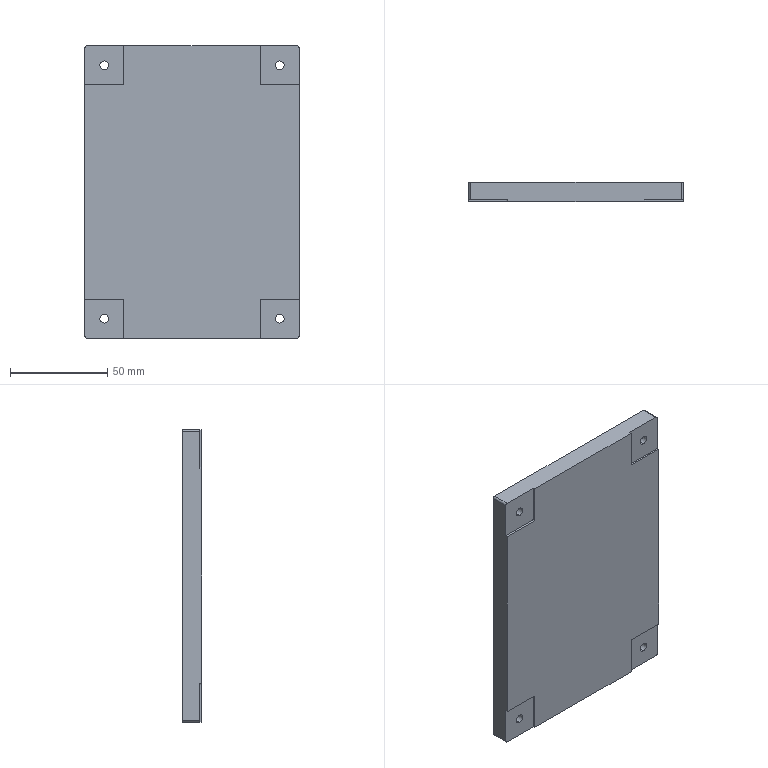Part | SolidWorks | features Fillet 2, Extrusion 1, HoleWzd 1, ICE 1 | 1 solid | 34 faces | box 110 x 10 x 150 mm | volume 162821 mm3 | plane 18 | cylinder 16 | commonest cylinder face diameters 2 x8 4.5 x8
STEP:
#1=CARTESIAN_POINT('',(45.,10.,-62.75));
#2=VERTEX_POINT('',#1);
#3=CARTESIAN_POINT('',(45.,10.,-67.25));
#4=VERTEX_POINT('',#3);
#5=CARTESIAN_POINT('',(45.,10.,-65.));
#6=DIRECTION('',(0.,-1.,0.));
#7=DIRECTION('',(0.,0.,-1.));
#8=AXIS2_PLACEMENT_3D('',#5,#6,#7);
#9=CIRCLE('',#8,2.25);
#10=EDGE_CURVE('',#2,#4,#9,.T.);
#11=ORIENTED_EDGE('',*,*,#10,.F.);
#12=CARTESIAN_POINT('',(45.,1.,-62.75));
#13=VERTEX_POINT('',#12);
#14=CARTESIAN_POINT('',(45.,1.,-62.75));
#15=DIRECTION('',(0.,-1.,0.));
#16=VECTOR('',#15,1000.);
#17=LINE('',#14,#16);
#18=EDGE_CURVE('',#2,#13,#17,.T.);
#19=ORIENTED_EDGE('',*,*,#18,.T.);
#20=CARTESIAN_POINT('',(45.,1.,-67.25));
#21=VERTEX_POINT('',#20);
#22=CARTESIAN_POINT('',(45.,1.,-65.));
#23=DIRECTION('',(0.,-1.,0.));
#24=DIRECTION('',(0.,0.,-1.));
#25=AXIS2_PLACEMENT_3D('',#22,#23,#24);
#26=CIRCLE('',#25,2.25);
#27=EDGE_CURVE('',#13,#21,#26,.T.);
#28=ORIENTED_EDGE('',*,*,#27,.T.);
#29=CARTESIAN_POINT('',(45.,1.,-67.25));
#30=DIRECTION('',(0.,-1.,0.));
#31=VECTOR('',#30,1000.);
#32=LINE('',#29,#31);
#33=EDGE_CURVE('',#4,#21,#32,.T.);
#34=ORIENTED_EDGE('',*,*,#33,.F.);
#35=EDGE_LOOP('',(#11,#19,#28,#34));
#36=FACE_OUTER_BOUND('',#35,.T.);
#37=CARTESIAN_POINT('',(45.,1.,-65.));
#38=DIRECTION('',(0.,-1.,0.));
#39=DIRECTION('',(0.,0.,-1.));
#40=AXIS2_PLACEMENT_3D('',#37,#38,#39);
#41=CYLINDRICAL_SURFACE('',#40,2.25);
#42=ADVANCED_FACE('',(#36),#41,.F.);
#43=CARTESIAN_POINT('',(-45.,10.,-62.75));
#44=VERTEX_POINT('',#43);
#45=CARTESIAN_POINT('',(-45.,10.,-67.25));
#46=VERTEX_POINT('',#45);
#47=CARTESIAN_POINT('',(-45.,10.,-65.));
#48=DIRECTION('',(0.,-1.,0.));
#49=DIRECTION('',(0.,0.,-1.));
#50=AXIS2_PLACEMENT_3D('',#47,#48,#49);
#51=CIRCLE('',#50,2.25);
#52=EDGE_CURVE('',#44,#46,#51,.T.);
#53=ORIENTED_EDGE('',*,*,#52,.F.);
#54=CARTESIAN_POINT('',(-45.,1.,-62.75));
#55=VERTEX_POINT('',#54);
#56=CARTESIAN_POINT('',(-45.,1.,-62.75));
#57=DIRECTION('',(0.,-1.,0.));
#58=VECTOR('',#57,1000.);
#59=LINE('',#56,#58);
#60=EDGE_CURVE('',#44,#55,#59,.T.);
#61=ORIENTED_EDGE('',*,*,#60,.T.);
#62=CARTESIAN_POINT('',(-45.,1.,-67.25));
#63=VERTEX_POINT('',#62);
#64=CARTESIAN_POINT('',(-45.,1.,-65.));
#65=DIRECTION('',(0.,-1.,0.));
#66=DIRECTION('',(0.,0.,-1.));
#67=AXIS2_PLACEMENT_3D('',#64,#65,#66);
#68=CIRCLE('',#67,2.25);
#69=EDGE_CURVE('',#55,#63,#68,.T.);
#70=ORIENTED_EDGE('',*,*,#69,.T.);
#71=CARTESIAN_POINT('',(-45.,1.,-67.25));
#72=DIRECTION('',(0.,-1.,0.));
#73=VECTOR('',#72,1000.);
#74=LINE('',#71,#73);
#75=EDGE_CURVE('',#46,#63,#74,.T.);
#76=ORIENTED_EDGE('',*,*,#75,.F.);
#77=EDGE_LOOP('',(#53,#61,#70,#76));
#78=FACE_OUTER_BOUND('',#77,.T.);
#79=CARTESIAN_POINT('',(-45.,1.,-65.));
#80=DIRECTION('',(0.,-1.,0.));
#81=DIRECTION('',(0.,0.,-1.));
#82=AXIS2_PLACEMENT_3D('',#79,#80,#81);
#83=CYLINDRICAL_SURFACE('',#82,2.25);
#84=ADVANCED_FACE('',(#78),#83,.F.);
#85=CARTESIAN_POINT('',(-45.,10.,67.25));
#86=VERTEX_POINT('',#85);
#87=CARTESIAN_POINT('',(-45.,10.,62.75));
#88=VERTEX_POINT('',#87);
#89=CARTESIAN_POINT('',(-45.,10.,65.));
#90=DIRECTION('',(0.,-1.,0.));
#91=DIRECTION('',(0.,0.,-1.));
#92=AXIS2_PLACEMENT_3D('',#89,#90,#91);
#93=CIRCLE('',#92,2.25);
#94=EDGE_CURVE('',#86,#88,#93,.T.);
#95=ORIENTED_EDGE('',*,*,#94,.F.);
#96=CARTESIAN_POINT('',(-45.,1.,67.25));
#97=VERTEX_POINT('',#96);
#98=CARTESIAN_POINT('',(-45.,1.,67.25));
#99=DIRECTION('',(0.,-1.,0.));
#100=VECTOR('',#99,1000.);
#101=LINE('',#98,#100);
#102=EDGE_CURVE('',#86,#97,#101,.T.);
#103=ORIENTED_EDGE('',*,*,#102,.T.);
#104=CARTESIAN_POINT('',(-45.,1.,62.75));
#105=VERTEX_POINT('',#104);
#106=CARTESIAN_POINT('',(-45.,1.,65.));
#107=DIRECTION('',(0.,-1.,0.));
#108=DIRECTION('',(0.,0.,-1.));
#109=AXIS2_PLACEMENT_3D('',#106,#107,#108);
#110=CIRCLE('',#109,2.25);
#111=EDGE_CURVE('',#97,#105,#110,.T.);
#112=ORIENTED_EDGE('',*,*,#111,.T.);
#113=CARTESIAN_POINT('',(-45.,1.,62.75));
#114=DIRECTION('',(0.,-1.,0.));
#115=VECTOR('',#114,1000.);
#116=LINE('',#113,#115);
#117=EDGE_CURVE('',#88,#105,#116,.T.);
#118=ORIENTED_EDGE('',*,*,#117,.F.);
#119=EDGE_LOOP('',(#95,#103,#112,#118));
#120=FACE_OUTER_BOUND('',#119,.T.);
#121=CARTESIAN_POINT('',(-45.,1.,65.));
#122=DIRECTION('',(0.,-1.,0.));
#123=DIRECTION('',(0.,0.,-1.));
#124=AXIS2_PLACEMENT_3D('',#121,#122,#123);
#125=CYLINDRICAL_SURFACE('',#124,2.25);
#126=ADVANCED_FACE('',(#120),#125,.F.);
#127=CARTESIAN_POINT('',(45.,10.,67.25));
#128=VERTEX_POINT('',#127);
#129=CARTESIAN_POINT('',(45.,10.,62.75));
#130=VERTEX_POINT('',#129);
#131=CARTESIAN_POINT('',(45.,10.,65.));
#132=DIRECTION('',(0.,-1.,0.));
#133=DIRECTION('',(0.,0.,-1.));
#134=AXIS2_PLACEMENT_3D('',#131,#132,#133);
#135=CIRCLE('',#134,2.25);
#136=EDGE_CURVE('',#128,#130,#135,.T.);
#137=ORIENTED_EDGE('',*,*,#136,.F.);
#138=CARTESIAN_POINT('',(45.,1.,67.25));
#139=VERTEX_POINT('',#138);
#140=CARTESIAN_POINT('',(45.,1.,67.25));
#141=DIRECTION('',(0.,-1.,0.));
#142=VECTOR('',#141,1000.);
#143=LINE('',#140,#142);
#144=EDGE_CURVE('',#128,#139,#143,.T.);
#145=ORIENTED_EDGE('',*,*,#144,.T.);
#146=CARTESIAN_POINT('',(45.,1.,62.75));
#147=VERTEX_POINT('',#146);
#148=CARTESIAN_POINT('',(45.,1.,65.));
#149=DIRECTION('',(0.,-1.,0.));
#150=DIRECTION('',(0.,0.,-1.));
#151=AXIS2_PLACEMENT_3D('',#148,#149,#150);
#152=CIRCLE('',#151,2.25);
#153=EDGE_CURVE('',#139,#147,#152,.T.);
#154=ORIENTED_EDGE('',*,*,#153,.T.);
#155=CARTESIAN_POINT('',(45.,1.,62.75));
#156=DIRECTION('',(0.,-1.,0.));
#157=VECTOR('',#156,1000.);
#158=LINE('',#155,#157);
#159=EDGE_CURVE('',#130,#147,#158,.T.);
#160=ORIENTED_EDGE('',*,*,#159,.F.);
#161=EDGE_LOOP('',(#137,#145,#154,#160));
#162=FACE_OUTER_BOUND('',#161,.T.);
#163=CARTESIAN_POINT('',(45.,1.,65.));
#164=DIRECTION('',(0.,-1.,0.));
#165=DIRECTION('',(0.,0.,-1.));
#166=AXIS2_PLACEMENT_3D('',#163,#164,#165);
#167=CYLINDRICAL_SURFACE('',#166,2.25);
#168=ADVANCED_FACE('',(#162),#167,.F.);
#169=CARTESIAN_POINT('',(-54.,10.,-75.));
#170=VERTEX_POINT('',#169);
#171=CARTESIAN_POINT('',(54.,10.,-75.));
#172=VERTEX_POINT('',#171);
#173=CARTESIAN_POINT('',(-55.,10.,-75.));
#174=DIRECTION('',(1.,0.,0.));
#175=VECTOR('',#174,1000.);
#176=LINE('',#173,#175);
#177=EDGE_CURVE('',#170,#172,#176,.T.);
#178=ORIENTED_EDGE('',*,*,#177,.T.);
#179=CARTESIAN_POINT('',(54.,1.,-75.));
#180=VERTEX_POINT('',#179);
#181=CARTESIAN_POINT('',(54.,10.,-75.));
#182=DIRECTION('',(0.,-1.,0.));
#183=VECTOR('',#182,1000.);
#184=LINE('',#181,#183);
#185=EDGE_CURVE('',#172,#180,#184,.T.);
#186=ORIENTED_EDGE('',*,*,#185,.T.);
#187=CARTESIAN_POINT('',(35.,1.,-75.));
#188=VERTEX_POINT('',#187);
#189=CARTESIAN_POINT('',(55.,1.,-75.));
#190=DIRECTION('',(1.,0.,0.));
#191=VECTOR('',#190,1000.);
#192=LINE('',#189,#191);
#193=EDGE_CURVE('',#188,#180,#192,.T.);
#194=ORIENTED_EDGE('',*,*,#193,.F.);
#195=CARTESIAN_POINT('',(35.,0.,-75.));
#196=VERTEX_POINT('',#195);
#197=CARTESIAN_POINT('',(35.,1.,-75.));
#198=DIRECTION('',(0.,-1.,0.));
#199=VECTOR('',#198,1000.);
#200=LINE('',#197,#199);
#201=EDGE_CURVE('',#188,#196,#200,.T.);
#202=ORIENTED_EDGE('',*,*,#201,.T.);
#203=CARTESIAN_POINT('',(-35.,0.,-75.));
#204=VERTEX_POINT('',#203);
#205=CARTESIAN_POINT('',(-55.,0.,-75.));
#206=DIRECTION('',(1.,0.,0.));
#207=VECTOR('',#206,1000.);
#208=LINE('',#205,#207);
#209=EDGE_CURVE('',#204,#196,#208,.T.);
#210=ORIENTED_EDGE('',*,*,#209,.F.);
#211=CARTESIAN_POINT('',(-35.,1.,-75.));
#212=VERTEX_POINT('',#211);
#213=CARTESIAN_POINT('',(-35.,1.,-75.));
#214=DIRECTION('',(0.,-1.,0.));
#215=VECTOR('',#214,1000.);
#216=LINE('',#213,#215);
#217=EDGE_CURVE('',#212,#204,#216,.T.);
#218=ORIENTED_EDGE('',*,*,#217,.F.);
#219=CARTESIAN_POINT('',(-54.,1.,-75.));
#220=VERTEX_POINT('',#219);
#221=CARTESIAN_POINT('',(-55.,1.,-75.));
#222=DIRECTION('',(1.,0.,0.));
#223=VECTOR('',#222,1000.);
#224=LINE('',#221,#223);
#225=EDGE_CURVE('',#220,#212,#224,.T.);
#226=ORIENTED_EDGE('',*,*,#225,.F.);
#227=CARTESIAN_POINT('',(-54.,10.,-75.));
#228=DIRECTION('',(0.,1.,0.));
#229=VECTOR('',#228,1000.);
#230=LINE('',#227,#229);
#231=EDGE_CURVE('',#220,#170,#230,.T.);
#232=ORIENTED_EDGE('',*,*,#231,.T.);
#233=EDGE_LOOP('',(#178,#186,#194,#202,#210,#218,#226,#232));
#234=FACE_OUTER_BOUND('',#233,.T.);
#235=CARTESIAN_POINT('',(-55.,10.,-75.));
#236=DIRECTION('',(0.,0.,-1.));
#237=DIRECTION('',(-1.,0.,0.));
#238=AXIS2_PLACEMENT_3D('',#235,#236,#237);
#239=PLANE('',#238);
#240=ADVANCED_FACE('',(#234),#239,.T.);
#241=CARTESIAN_POINT('',(-55.,1.,74.));
#242=VERTEX_POINT('',#241);
#243=CARTESIAN_POINT('',(-55.,1.,55.));
#244=VERTEX_POINT('',#243);
#245=CARTESIAN_POINT('',(-55.,1.,75.));
#246=DIRECTION('',(0.,0.,-1.));
#247=VECTOR('',#246,1000.);
#248=LINE('',#245,#247);
#249=EDGE_CURVE('',#242,#244,#248,.T.);
#250=ORIENTED_EDGE('',*,*,#249,.F.);
#251=CARTESIAN_POINT('',(-55.,10.,74.));
#252=VERTEX_POINT('',#251);
#253=CARTESIAN_POINT('',(-55.,10.,74.));
#254=DIRECTION('',(0.,1.,0.));
#255=VECTOR('',#254,1000.);
#256=LINE('',#253,#255);
#257=EDGE_CURVE('',#242,#252,#256,.T.);
#258=ORIENTED_EDGE('',*,*,#257,.T.);
#259=CARTESIAN_POINT('',(-55.,10.,-74.));
#260=VERTEX_POINT('',#259);
#261=CARTESIAN_POINT('',(-55.,10.,-75.));
#262=DIRECTION('',(0.,0.,1.));
#263=VECTOR('',#262,1000.);
#264=LINE('',#261,#263);
#265=EDGE_CURVE('',#260,#252,#264,.T.);
#266=ORIENTED_EDGE('',*,*,#265,.F.);
#267=CARTESIAN_POINT('',(-55.,1.,-74.));
#268=VERTEX_POINT('',#267);
#269=CARTESIAN_POINT('',(-55.,1.,-74.));
#270=DIRECTION('',(0.,-1.,0.));
#271=VECTOR('',#270,1000.);
#272=LINE('',#269,#271);
#273=EDGE_CURVE('',#260,#268,#272,.T.);
#274=ORIENTED_EDGE('',*,*,#273,.T.);
#275=CARTESIAN_POINT('',(-55.,1.,-55.));
#276=VERTEX_POINT('',#275);
#277=CARTESIAN_POINT('',(-55.,1.,-75.));
#278=DIRECTION('',(0.,0.,-1.));
#279=VECTOR('',#278,1000.);
#280=LINE('',#277,#279);
#281=EDGE_CURVE('',#276,#268,#280,.T.);
#282=ORIENTED_EDGE('',*,*,#281,.F.);
#283=CARTESIAN_POINT('',(-55.,0.,-55.));
#284=VERTEX_POINT('',#283);
#285=CARTESIAN_POINT('',(-55.,1.,-55.));
#286=DIRECTION('',(0.,-1.,0.));
#287=VECTOR('',#286,1000.);
#288=LINE('',#285,#287);
#289=EDGE_CURVE('',#276,#284,#288,.T.);
#290=ORIENTED_EDGE('',*,*,#289,.T.);
#291=CARTESIAN_POINT('',(-55.,0.,55.));
#292=VERTEX_POINT('',#291);
#293=CARTESIAN_POINT('',(-55.,0.,-75.));
#294=DIRECTION('',(0.,0.,1.));
#295=VECTOR('',#294,1000.);
#296=LINE('',#293,#295);
#297=EDGE_CURVE('',#284,#292,#296,.T.);
#298=ORIENTED_EDGE('',*,*,#297,.T.);
#299=CARTESIAN_POINT('',(-55.,1.,55.));
#300=DIRECTION('',(0.,-1.,0.));
#301=VECTOR('',#300,1000.);
#302=LINE('',#299,#301);
#303=EDGE_CURVE('',#244,#292,#302,.T.);
#304=ORIENTED_EDGE('',*,*,#303,.F.);
#305=EDGE_LOOP('',(#250,#258,#266,#274,#282,#290,#298,#304));
#306=FACE_OUTER_BOUND('',#305,.T.);
#307=CARTESIAN_POINT('',(-55.,10.,-75.));
#308=DIRECTION('',(1.,0.,0.));
#309=DIRECTION('',(0.,0.,-1.));
#310=AXIS2_PLACEMENT_3D('',#307,#308,#309);
#311=PLANE('',#310);
#312=ADVANCED_FACE('',(#306),#311,.F.);
#313=CARTESIAN_POINT('',(54.,1.,75.));
#314=VERTEX_POINT('',#313);
#315=CARTESIAN_POINT('',(35.,1.,75.));
#316=VERTEX_POINT('',#315);
#317=CARTESIAN_POINT('',(55.,1.,75.));
#318=DIRECTION('',(-1.,0.,0.));
#319=VECTOR('',#318,1000.);
#320=LINE('',#317,#319);
#321=EDGE_CURVE('',#314,#316,#320,.T.);
#322=ORIENTED_EDGE('',*,*,#321,.F.);
#323=CARTESIAN_POINT('',(54.,10.,75.));
#324=VERTEX_POINT('',#323);
#325=CARTESIAN_POINT('',(54.,10.,75.));
#326=DIRECTION('',(0.,1.,0.));
#327=VECTOR('',#326,1000.);
#328=LINE('',#325,#327);
#329=EDGE_CURVE('',#314,#324,#328,.T.);
#330=ORIENTED_EDGE('',*,*,#329,.T.);
#331=CARTESIAN_POINT('',(-54.,10.,75.));
#332=VERTEX_POINT('',#331);
#333=CARTESIAN_POINT('',(-55.,10.,75.));
#334=DIRECTION('',(1.,0.,0.));
#335=VECTOR('',#334,1000.);
#336=LINE('',#333,#335);
#337=EDGE_CURVE('',#332,#324,#336,.T.);
#338=ORIENTED_EDGE('',*,*,#337,.F.);
#339=CARTESIAN_POINT('',(-54.,1.,75.));
#340=VERTEX_POINT('',#339);
#341=CARTESIAN_POINT('',(-54.,10.,75.));
#342=DIRECTION('',(0.,-1.,0.));
#343=VECTOR('',#342,1000.);
#344=LINE('',#341,#343);
#345=EDGE_CURVE('',#332,#340,#344,.T.);
#346=ORIENTED_EDGE('',*,*,#345,.T.);
#347=CARTESIAN_POINT('',(-35.,1.,75.));
#348=VERTEX_POINT('',#347);
#349=CARTESIAN_POINT('',(-55.,1.,75.));
#350=DIRECTION('',(-1.,0.,0.));
#351=VECTOR('',#350,1000.);
#352=LINE('',#349,#351);
#353=EDGE_CURVE('',#348,#340,#352,.T.);
#354=ORIENTED_EDGE('',*,*,#353,.F.);
#355=CARTESIAN_POINT('',(-35.,0.,75.));
#356=VERTEX_POINT('',#355);
#357=CARTESIAN_POINT('',(-35.,1.,75.));
#358=DIRECTION('',(0.,-1.,0.));
#359=VECTOR('',#358,1000.);
#360=LINE('',#357,#359);
#361=EDGE_CURVE('',#348,#356,#360,.T.);
#362=ORIENTED_EDGE('',*,*,#361,.T.);
#363=CARTESIAN_POINT('',(35.,0.,75.));
#364=VERTEX_POINT('',#363);
#365=CARTESIAN_POINT('',(-55.,0.,75.));
#366=DIRECTION('',(1.,0.,0.));
#367=VECTOR('',#366,1000.);
#368=LINE('',#365,#367);
#369=EDGE_CURVE('',#356,#364,#368,.T.);
#370=ORIENTED_EDGE('',*,*,#369,.T.);
#371=CARTESIAN_POINT('',(35.,1.,75.));
#372=DIRECTION('',(0.,-1.,0.));
#373=VECTOR('',#372,1000.);
#374=LINE('',#371,#373);
#375=EDGE_CURVE('',#316,#364,#374,.T.);
#376=ORIENTED_EDGE('',*,*,#375,.F.);
#377=EDGE_LOOP('',(#322,#330,#338,#346,#354,#362,#370,#376));
#378=FACE_OUTER_BOUND('',#377,.T.);
#379=CARTESIAN_POINT('',(-55.,10.,75.));
#380=DIRECTION('',(0.,0.,-1.));
#381=DIRECTION('',(-1.,0.,0.));
#382=AXIS2_PLACEMENT_3D('',#379,#380,#381);
#383=PLANE('',#382);
#384=ADVANCED_FACE('',(#378),#383,.F.);
#385=CARTESIAN_POINT('',(55.,1.,-74.));
#386=VERTEX_POINT('',#385);
#387=CARTESIAN_POINT('',(55.,1.,-55.));
#388=VERTEX_POINT('',#387);
#389=CARTESIAN_POINT('',(55.,1.,-75.));
#390=DIRECTION('',(0.,0.,1.));
#391=VECTOR('',#390,1000.);
#392=LINE('',#389,#391);
#393=EDGE_CURVE('',#386,#388,#392,.T.);
#394=ORIENTED_EDGE('',*,*,#393,.F.);
#395=CARTESIAN_POINT('',(55.,10.,-74.));
#396=VERTEX_POINT('',#395);
#397=CARTESIAN_POINT('',(55.,10.,-74.));
#398=DIRECTION('',(0.,1.,0.));
#399=VECTOR('',#398,1000.);
#400=LINE('',#397,#399);
#401=EDGE_CURVE('',#386,#396,#400,.T.);
#402=ORIENTED_EDGE('',*,*,#401,.T.);
#403=CARTESIAN_POINT('',(55.,10.,74.));
#404=VERTEX_POINT('',#403);
#405=CARTESIAN_POINT('',(55.,10.,-75.));
#406=DIRECTION('',(0.,0.,1.));
#407=VECTOR('',#406,1000.);
#408=LINE('',#405,#407);
#409=EDGE_CURVE('',#396,#404,#408,.T.);
#410=ORIENTED_EDGE('',*,*,#409,.T.);
#411=CARTESIAN_POINT('',(55.,1.,74.));
#412=VERTEX_POINT('',#411);
#413=CARTESIAN_POINT('',(55.,1.,74.));
#414=DIRECTION('',(0.,-1.,0.));
#415=VECTOR('',#414,1000.);
#416=LINE('',#413,#415);
#417=EDGE_CURVE('',#404,#412,#416,.T.);
#418=ORIENTED_EDGE('',*,*,#417,.T.);
#419=CARTESIAN_POINT('',(55.,1.,55.));
#420=VERTEX_POINT('',#419);
#421=CARTESIAN_POINT('',(55.,1.,75.));
#422=DIRECTION('',(0.,0.,1.));
#423=VECTOR('',#422,1000.);
#424=LINE('',#421,#423);
#425=EDGE_CURVE('',#420,#412,#424,.T.);
#426=ORIENTED_EDGE('',*,*,#425,.F.);
#427=CARTESIAN_POINT('',(55.,0.,55.));
#428=VERTEX_POINT('',#427);
#429=CARTESIAN_POINT('',(55.,1.,55.));
#430=DIRECTION('',(0.,-1.,0.));
#431=VECTOR('',#430,1000.);
#432=LINE('',#429,#431);
#433=EDGE_CURVE('',#420,#428,#432,.T.);
#434=ORIENTED_EDGE('',*,*,#433,.T.);
#435=CARTESIAN_POINT('',(55.,0.,-55.));
#436=VERTEX_POINT('',#435);
#437=CARTESIAN_POINT('',(55.,0.,-75.));
#438=DIRECTION('',(0.,0.,1.));
#439=VECTOR('',#438,1000.);
#440=LINE('',#437,#439);
#441=EDGE_CURVE('',#436,#428,#440,.T.);
#442=ORIENTED_EDGE('',*,*,#441,.F.);
#443=CARTESIAN_POINT('',(55.,1.,-55.));
#444=DIRECTION('',(0.,-1.,0.));
#445=VECTOR('',#444,1000.);
#446=LINE('',#443,#445);
#447=EDGE_CURVE('',#388,#436,#446,.T.);
#448=ORIENTED_EDGE('',*,*,#447,.F.);
#449=EDGE_LOOP('',(#394,#402,#410,#418,#426,#434,#442,#448));
#450=FACE_OUTER_BOUND('',#449,.T.);
#451=CARTESIAN_POINT('',(55.,10.,-75.));
#452=DIRECTION('',(1.,0.,0.));
#453=DIRECTION('',(0.,0.,-1.));
#454=AXIS2_PLACEMENT_3D('',#451,#452,#453);
#455=PLANE('',#454);
#456=ADVANCED_FACE('',(#450),#455,.T.);
#457=CARTESIAN_POINT('',(45.,10.,-65.));
#458=DIRECTION('',(0.,-1.,0.));
#459=DIRECTION('',(0.,0.,-1.));
#460=AXIS2_PLACEMENT_3D('',#457,#458,#459);
#461=CIRCLE('',#460,2.25);
#462=EDGE_CURVE('',#4,#2,#461,.T.);
#463=ORIENTED_EDGE('',*,*,#462,.T.);
#464=ORIENTED_EDGE('',*,*,#10,.T.);
#465=EDGE_LOOP('',(#463,#464));
#466=FACE_BOUND('',#465,.T.);
#467=CARTESIAN_POINT('',(-45.,10.,-65.));
#468=DIRECTION('',(0.,-1.,0.));
#469=DIRECTION('',(0.,0.,-1.));
#470=AXIS2_PLACEMENT_3D('',#467,#468,#469);
#471=CIRCLE('',#470,2.25);
#472=EDGE_CURVE('',#46,#44,#471,.T.);
#473=ORIENTED_EDGE('',*,*,#472,.T.);
#474=ORIENTED_EDGE('',*,*,#52,.T.);
#475=EDGE_LOOP('',(#473,#474));
#476=FACE_BOUND('',#475,.T.);
#477=CARTESIAN_POINT('',(-45.,10.,65.));
#478=DIRECTION('',(0.,-1.,0.));
#479=DIRECTION('',(0.,0.,-1.));
#480=AXIS2_PLACEMENT_3D('',#477,#478,#479);
#481=CIRCLE('',#480,2.25);
#482=EDGE_CURVE('',#88,#86,#481,.T.);
#483=ORIENTED_EDGE('',*,*,#482,.T.);
#484=ORIENTED_EDGE('',*,*,#94,.T.);
#485=EDGE_LOOP('',(#483,#484));
#486=FACE_BOUND('',#485,.T.);
#487=CARTESIAN_POINT('',(45.,10.,65.));
#488=DIRECTION('',(0.,-1.,0.));
#489=DIRECTION('',(0.,0.,-1.));
#490=AXIS2_PLACEMENT_3D('',#487,#488,#489);
#491=CIRCLE('',#490,2.25);
#492=EDGE_CURVE('',#130,#128,#491,.T.);
#493=ORIENTED_EDGE('',*,*,#492,.T.);
#494=ORIENTED_EDGE('',*,*,#136,.T.);
#495=EDGE_LOOP('',(#493,#494));
#496=FACE_BOUND('',#495,.T.);
#497=ORIENTED_EDGE('',*,*,#409,.F.);
#498=CARTESIAN_POINT('',(54.,10.,-74.));
#499=DIRECTION('',(0.,1.,0.));
#500=DIRECTION('',(0.,0.,-1.));
#501=AXIS2_PLACEMENT_3D('',#498,#499,#500);
#502=CIRCLE('',#501,1.);
#503=EDGE_CURVE('',#396,#172,#502,.T.);
#504=ORIENTED_EDGE('',*,*,#503,.T.);
#505=ORIENTED_EDGE('',*,*,#177,.F.);
#506=CARTESIAN_POINT('',(-54.,10.,-74.));
#507=DIRECTION('',(0.,1.,0.));
#508=DIRECTION('',(0.,0.,-1.));
#509=AXIS2_PLACEMENT_3D('',#506,#507,#508);
#510=CIRCLE('',#509,1.);
#511=EDGE_CURVE('',#170,#260,#510,.T.);
#512=ORIENTED_EDGE('',*,*,#511,.T.);
#513=ORIENTED_EDGE('',*,*,#265,.T.);
#514=CARTESIAN_POINT('',(-54.,10.,74.));
#515=DIRECTION('',(0.,1.,0.));
#516=DIRECTION('',(0.,0.,-1.));
#517=AXIS2_PLACEMENT_3D('',#514,#515,#516);
#518=CIRCLE('',#517,1.);
#519=EDGE_CURVE('',#252,#332,#518,.T.);
#520=ORIENTED_EDGE('',*,*,#519,.T.);
#521=ORIENTED_EDGE('',*,*,#337,.T.);
#522=CARTESIAN_POINT('',(54.,10.,74.));
#523=DIRECTION('',(0.,1.,0.));
#524=DIRECTION('',(0.,0.,-1.));
#525=AXIS2_PLACEMENT_3D('',#522,#523,#524);
#526=CIRCLE('',#525,1.);
#527=EDGE_CURVE('',#324,#404,#526,.T.);
#528=ORIENTED_EDGE('',*,*,#527,.T.);
#529=EDGE_LOOP('',(#497,#504,#505,#512,#513,#520,#521,#528));
#530=FACE_OUTER_BOUND('',#529,.T.);
#531=CARTESIAN_POINT('',(0.,10.,0.));
#532=DIRECTION('',(0.,-1.,0.));
#533=DIRECTION('',(0.,0.,-1.));
#534=AXIS2_PLACEMENT_3D('',#531,#532,#533);
#535=PLANE('',#534);
#536=ADVANCED_FACE('',(#466,#476,#486,#496,#530),#535,.F.);
#537=CARTESIAN_POINT('',(-36.,0.,-55.));
#538=VERTEX_POINT('',#537);
#539=CARTESIAN_POINT('',(-55.,0.,-55.));
#540=DIRECTION('',(-1.,0.,0.));
#541=VECTOR('',#540,1000.);
#542=LINE('',#539,#541);
#543=EDGE_CURVE('',#538,#284,#542,.T.);
#544=ORIENTED_EDGE('',*,*,#543,.F.);
#545=CARTESIAN_POINT('',(-35.,0.,-56.));
#546=VERTEX_POINT('',#545);
#547=CARTESIAN_POINT('',(-36.,0.,-56.));
#548=DIRECTION('',(0.,1.,0.));
#549=DIRECTION('',(0.,0.,-1.));
#550=AXIS2_PLACEMENT_3D('',#547,#548,#549);
#551=CIRCLE('',#550,1.);
#552=EDGE_CURVE('',#538,#546,#551,.T.);
#553=ORIENTED_EDGE('',*,*,#552,.T.);
#554=CARTESIAN_POINT('',(-35.,0.,-75.));
#555=DIRECTION('',(0.,0.,1.));
#556=VECTOR('',#555,1000.);
#557=LINE('',#554,#556);
#558=EDGE_CURVE('',#204,#546,#557,.T.);
#559=ORIENTED_EDGE('',*,*,#558,.F.);
#560=ORIENTED_EDGE('',*,*,#209,.T.);
#561=CARTESIAN_POINT('',(35.,0.,-56.));
#562=VERTEX_POINT('',#561);
#563=CARTESIAN_POINT('',(35.,0.,-75.));
#564=DIRECTION('',(0.,0.,-1.));
#565=VECTOR('',#564,1000.);
#566=LINE('',#563,#565);
#567=EDGE_CURVE('',#562,#196,#566,.T.);
#568=ORIENTED_EDGE('',*,*,#567,.F.);
#569=CARTESIAN_POINT('',(36.,0.,-55.));
#570=VERTEX_POINT('',#569);
#571=CARTESIAN_POINT('',(36.,0.,-56.));
#572=DIRECTION('',(0.,1.,0.));
#573=DIRECTION('',(0.,0.,-1.));
#574=AXIS2_PLACEMENT_3D('',#571,#572,#573);
#575=CIRCLE('',#574,1.);
#576=EDGE_CURVE('',#562,#570,#575,.T.);
#577=ORIENTED_EDGE('',*,*,#576,.T.);
#578=CARTESIAN_POINT('',(55.,0.,-55.));
#579=DIRECTION('',(-1.,0.,0.));
#580=VECTOR('',#579,1000.);
#581=LINE('',#578,#580);
#582=EDGE_CURVE('',#436,#570,#581,.T.);
#583=ORIENTED_EDGE('',*,*,#582,.F.);
#584=ORIENTED_EDGE('',*,*,#441,.T.);
#585=CARTESIAN_POINT('',(36.,0.,55.));
#586=VERTEX_POINT('',#585);
#587=CARTESIAN_POINT('',(55.,0.,55.));
#588=DIRECTION('',(1.,0.,0.));
#589=VECTOR('',#588,1000.);
#590=LINE('',#587,#589);
#591=EDGE_CURVE('',#586,#428,#590,.T.);
#592=ORIENTED_EDGE('',*,*,#591,.F.);
#593=CARTESIAN_POINT('',(35.,0.,56.));
#594=VERTEX_POINT('',#593);
#595=CARTESIAN_POINT('',(36.,0.,56.));
#596=DIRECTION('',(0.,1.,0.));
#597=DIRECTION('',(0.,0.,-1.));
#598=AXIS2_PLACEMENT_3D('',#595,#596,#597);
#599=CIRCLE('',#598,1.);
#600=EDGE_CURVE('',#586,#594,#599,.T.);
#601=ORIENTED_EDGE('',*,*,#600,.T.);
#602=CARTESIAN_POINT('',(35.,0.,75.));
#603=DIRECTION('',(0.,0.,-1.));
#604=VECTOR('',#603,1000.);
#605=LINE('',#602,#604);
#606=EDGE_CURVE('',#364,#594,#605,.T.);
#607=ORIENTED_EDGE('',*,*,#606,.F.);
#608=ORIENTED_EDGE('',*,*,#369,.F.);
#609=CARTESIAN_POINT('',(-35.,0.,56.));
#610=VERTEX_POINT('',#609);
#611=CARTESIAN_POINT('',(-35.,0.,75.));
#612=DIRECTION('',(0.,0.,1.));
#613=VECTOR('',#612,1000.);
#614=LINE('',#611,#613);
#615=EDGE_CURVE('',#610,#356,#614,.T.);
#616=ORIENTED_EDGE('',*,*,#615,.F.);
#617=CARTESIAN_POINT('',(-36.,0.,55.));
#618=VERTEX_POINT('',#617);
#619=CARTESIAN_POINT('',(-36.,0.,56.));
#620=DIRECTION('',(0.,1.,0.));
#621=DIRECTION('',(0.,0.,-1.));
#622=AXIS2_PLACEMENT_3D('',#619,#620,#621);
#623=CIRCLE('',#622,1.);
#624=EDGE_CURVE('',#610,#618,#623,.T.);
#625=ORIENTED_EDGE('',*,*,#624,.T.);
#626=CARTESIAN_POINT('',(-55.,0.,55.));
#627=DIRECTION('',(1.,0.,0.));
#628=VECTOR('',#627,1000.);
#629=LINE('',#626,#628);
#630=EDGE_CURVE('',#292,#618,#629,.T.);
#631=ORIENTED_EDGE('',*,*,#630,.F.);
#632=ORIENTED_EDGE('',*,*,#297,.F.);
#633=EDGE_LOOP('',(#544,#553,#559,#560,#568,#577,#583,#584,#592,#601,#607,#608,#616,#625,#631,#632));
#634=FACE_OUTER_BOUND('',#633,.T.);
#635=CARTESIAN_POINT('',(0.,0.,0.));
#636=DIRECTION('',(0.,-1.,0.));
#637=DIRECTION('',(0.,0.,-1.));
#638=AXIS2_PLACEMENT_3D('',#635,#636,#637);
#639=PLANE('',#638);
#640=ADVANCED_FACE('',(#634),#639,.T.);
#641=CARTESIAN_POINT('',(-35.,1.,56.));
#642=VERTEX_POINT('',#641);
#643=CARTESIAN_POINT('',(-35.,1.,75.));
#644=DIRECTION('',(0.,0.,1.));
#645=VECTOR('',#644,1000.);
#646=LINE('',#643,#645);
#647=EDGE_CURVE('',#642,#348,#646,.T.);
#648=ORIENTED_EDGE('',*,*,#647,.F.);
#649=CARTESIAN_POINT('',(-35.,0.,56.));
#650=DIRECTION('',(0.,-1.,0.));
#651=VECTOR('',#650,1000.);
#652=LINE('',#649,#651);
#653=EDGE_CURVE('',#642,#610,#652,.T.);
#654=ORIENTED_EDGE('',*,*,#653,.T.);
#655=ORIENTED_EDGE('',*,*,#615,.T.);
#656=ORIENTED_EDGE('',*,*,#361,.F.);
#657=EDGE_LOOP('',(#648,#654,#655,#656));
#658=FACE_OUTER_BOUND('',#657,.T.);
#659=CARTESIAN_POINT('',(-35.,1.,75.));
#660=DIRECTION('',(1.,0.,0.));
#661=DIRECTION('',(0.,0.,-1.));
#662=AXIS2_PLACEMENT_3D('',#659,#660,#661);
#663=PLANE('',#662);
#664=ADVANCED_FACE('',(#658),#663,.F.);
#665=ORIENTED_EDGE('',*,*,#630,.T.);
#666=CARTESIAN_POINT('',(-36.,1.,55.));
#667=VERTEX_POINT('',#666);
#668=CARTESIAN_POINT('',(-36.,1.,55.));
#669=DIRECTION('',(0.,1.,0.));
#670=VECTOR('',#669,1000.);
#671=LINE('',#668,#670);
#672=EDGE_CURVE('',#618,#667,#671,.T.);
#673=ORIENTED_EDGE('',*,*,#672,.T.);
#674=CARTESIAN_POINT('',(-55.,1.,55.));
#675=DIRECTION('',(1.,0.,0.));
#676=VECTOR('',#675,1000.);
#677=LINE('',#674,#676);
#678=EDGE_CURVE('',#244,#667,#677,.T.);
#679=ORIENTED_EDGE('',*,*,#678,.F.);
#680=ORIENTED_EDGE('',*,*,#303,.T.);
#681=EDGE_LOOP('',(#665,#673,#679,#680));
#682=FACE_OUTER_BOUND('',#681,.T.);
#683=CARTESIAN_POINT('',(-55.,1.,55.));
#684=DIRECTION('',(0.,0.,-1.));
#685=DIRECTION('',(-1.,0.,0.));
#686=AXIS2_PLACEMENT_3D('',#683,#684,#685);
#687=PLANE('',#686);
#688=ADVANCED_FACE('',(#682),#687,.F.);
#689=CARTESIAN_POINT('',(-45.,1.,65.));
#690=DIRECTION('',(0.,-1.,0.));
#691=DIRECTION('',(0.,0.,-1.));
#692=AXIS2_PLACEMENT_3D('',#689,#690,#691);
#693=CIRCLE('',#692,2.25);
#694=EDGE_CURVE('',#105,#97,#693,.T.);
#695=ORIENTED_EDGE('',*,*,#694,.F.);
#696=ORIENTED_EDGE('',*,*,#111,.F.);
#697=EDGE_LOOP('',(#695,#696));
#698=FACE_BOUND('',#697,.T.);
#699=ORIENTED_EDGE('',*,*,#353,.T.);
#700=CARTESIAN_POINT('',(-54.,1.,74.));
#701=DIRECTION('',(0.,-1.,0.));
#702=DIRECTION('',(0.,0.,-1.));
#703=AXIS2_PLACEMENT_3D('',#700,#701,#702);
#704=CIRCLE('',#703,1.);
#705=EDGE_CURVE('',#340,#242,#704,.T.);
#706=ORIENTED_EDGE('',*,*,#705,.T.);
#707=ORIENTED_EDGE('',*,*,#249,.T.);
#708=ORIENTED_EDGE('',*,*,#678,.T.);
#709=CARTESIAN_POINT('',(-36.,1.,56.));
#710=DIRECTION('',(0.,-1.,0.));
#711=DIRECTION('',(0.,0.,-1.));
#712=AXIS2_PLACEMENT_3D('',#709,#710,#711);
#713=CIRCLE('',#712,1.);
#714=EDGE_CURVE('',#667,#642,#713,.T.);
#715=ORIENTED_EDGE('',*,*,#714,.T.);
#716=ORIENTED_EDGE('',*,*,#647,.T.);
#717=EDGE_LOOP('',(#699,#706,#707,#708,#715,#716));
#718=FACE_OUTER_BOUND('',#717,.T.);
#719=CARTESIAN_POINT('',(0.,1.,0.));
#720=DIRECTION('',(0.,-1.,0.));
#721=DIRECTION('',(0.,0.,-1.));
#722=AXIS2_PLACEMENT_3D('',#719,#720,#721);
#723=PLANE('',#722);
#724=ADVANCED_FACE('',(#698,#718),#723,.T.);
#725=CARTESIAN_POINT('',(36.,1.,55.));
#726=VERTEX_POINT('',#725);
#727=CARTESIAN_POINT('',(55.,1.,55.));
#728=DIRECTION('',(1.,0.,0.));
#729=VECTOR('',#728,1000.);
#730=LINE('',#727,#729);
#731=EDGE_CURVE('',#726,#420,#730,.T.);
#732=ORIENTED_EDGE('',*,*,#731,.F.);
#733=CARTESIAN_POINT('',(36.,0.,55.));
#734=DIRECTION('',(0.,-1.,0.));
#735=VECTOR('',#734,1000.);
#736=LINE('',#733,#735);
#737=EDGE_CURVE('',#726,#586,#736,.T.);
#738=ORIENTED_EDGE('',*,*,#737,.T.);
#739=ORIENTED_EDGE('',*,*,#591,.T.);
#740=ORIENTED_EDGE('',*,*,#433,.F.);
#741=EDGE_LOOP('',(#732,#738,#739,#740));
#742=FACE_OUTER_BOUND('',#741,.T.);
#743=CARTESIAN_POINT('',(55.,1.,55.));
#744=DIRECTION('',(0.,0.,-1.));
#745=DIRECTION('',(-1.,0.,0.));
#746=AXIS2_PLACEMENT_3D('',#743,#744,#745);
#747=PLANE('',#746);
#748=ADVANCED_FACE('',(#742),#747,.F.);
#749=ORIENTED_EDGE('',*,*,#606,.T.);
#750=CARTESIAN_POINT('',(35.,1.,56.));
#751=VERTEX_POINT('',#750);
#752=CARTESIAN_POINT('',(35.,1.,56.));
#753=DIRECTION('',(0.,1.,0.));
#754=VECTOR('',#753,1000.);
#755=LINE('',#752,#754);
#756=EDGE_CURVE('',#594,#751,#755,.T.);
#757=ORIENTED_EDGE('',*,*,#756,.T.);
#758=CARTESIAN_POINT('',(35.,1.,75.));
#759=DIRECTION('',(0.,0.,-1.));
#760=VECTOR('',#759,1000.);
#761=LINE('',#758,#760);
#762=EDGE_CURVE('',#316,#751,#761,.T.);
#763=ORIENTED_EDGE('',*,*,#762,.F.);
#764=ORIENTED_EDGE('',*,*,#375,.T.);
#765=EDGE_LOOP('',(#749,#757,#763,#764));
#766=FACE_OUTER_BOUND('',#765,.T.);
#767=CARTESIAN_POINT('',(35.,1.,75.));
#768=DIRECTION('',(-1.,0.,0.));
#769=DIRECTION('',(0.,0.,1.));
#770=AXIS2_PLACEMENT_3D('',#767,#768,#769);
#771=PLANE('',#770);
#772=ADVANCED_FACE('',(#766),#771,.F.);
#773=CARTESIAN_POINT('',(45.,1.,65.));
#774=DIRECTION('',(0.,-1.,0.));
#775=DIRECTION('',(0.,0.,-1.));
#776=AXIS2_PLACEMENT_3D('',#773,#774,#775);
#777=CIRCLE('',#776,2.25);
#778=EDGE_CURVE('',#147,#139,#777,.T.);
#779=ORIENTED_EDGE('',*,*,#778,.F.);
#780=ORIENTED_EDGE('',*,*,#153,.F.);
#781=EDGE_LOOP('',(#779,#780));
#782=FACE_BOUND('',#781,.T.);
#783=ORIENTED_EDGE('',*,*,#425,.T.);
#784=CARTESIAN_POINT('',(54.,1.,74.));
#785=DIRECTION('',(0.,-1.,0.));
#786=DIRECTION('',(0.,0.,1.));
#787=AXIS2_PLACEMENT_3D('',#784,#785,#786);
#788=CIRCLE('',#787,1.);
#789=EDGE_CURVE('',#412,#314,#788,.T.);
#790=ORIENTED_EDGE('',*,*,#789,.T.);
#791=ORIENTED_EDGE('',*,*,#321,.T.);
#792=ORIENTED_EDGE('',*,*,#762,.T.);
#793=CARTESIAN_POINT('',(36.,1.,56.));
#794=DIRECTION('',(0.,-1.,0.));
#795=DIRECTION('',(0.,0.,1.));
#796=AXIS2_PLACEMENT_3D('',#793,#794,#795);
#797=CIRCLE('',#796,1.);
#798=EDGE_CURVE('',#751,#726,#797,.T.);
#799=ORIENTED_EDGE('',*,*,#798,.T.);
#800=ORIENTED_EDGE('',*,*,#731,.T.);
#801=EDGE_LOOP('',(#783,#790,#791,#792,#799,#800));
#802=FACE_OUTER_BOUND('',#801,.T.);
#803=CARTESIAN_POINT('',(0.,1.,0.));
#804=DIRECTION('',(0.,1.,0.));
#805=DIRECTION('',(0.,0.,1.));
#806=AXIS2_PLACEMENT_3D('',#803,#804,#805);
#807=PLANE('',#806);
#808=ADVANCED_FACE('',(#782,#802),#807,.F.);
#809=CARTESIAN_POINT('',(35.,1.,-56.));
#810=VERTEX_POINT('',#809);
#811=CARTESIAN_POINT('',(35.,1.,-75.));
#812=DIRECTION('',(0.,0.,-1.));
#813=VECTOR('',#812,1000.);
#814=LINE('',#811,#813);
#815=EDGE_CURVE('',#810,#188,#814,.T.);
#816=ORIENTED_EDGE('',*,*,#815,.F.);
#817=CARTESIAN_POINT('',(35.,0.,-56.));
#818=DIRECTION('',(0.,-1.,0.));
#819=VECTOR('',#818,1000.);
#820=LINE('',#817,#819);
#821=EDGE_CURVE('',#810,#562,#820,.T.);
#822=ORIENTED_EDGE('',*,*,#821,.T.);
#823=ORIENTED_EDGE('',*,*,#567,.T.);
#824=ORIENTED_EDGE('',*,*,#201,.F.);
#825=EDGE_LOOP('',(#816,#822,#823,#824));
#826=FACE_OUTER_BOUND('',#825,.T.);
#827=CARTESIAN_POINT('',(35.,1.,-75.));
#828=DIRECTION('',(-1.,0.,0.));
#829=DIRECTION('',(0.,0.,1.));
#830=AXIS2_PLACEMENT_3D('',#827,#828,#829);
#831=PLANE('',#830);
#832=ADVANCED_FACE('',(#826),#831,.F.);
#833=ORIENTED_EDGE('',*,*,#582,.T.);
#834=CARTESIAN_POINT('',(36.,1.,-55.));
#835=VERTEX_POINT('',#834);
#836=CARTESIAN_POINT('',(36.,1.,-55.));
#837=DIRECTION('',(0.,1.,0.));
#838=VECTOR('',#837,1000.);
#839=LINE('',#836,#838);
#840=EDGE_CURVE('',#570,#835,#839,.T.);
#841=ORIENTED_EDGE('',*,*,#840,.T.);
#842=CARTESIAN_POINT('',(55.,1.,-55.));
#843=DIRECTION('',(-1.,0.,0.));
#844=VECTOR('',#843,1000.);
#845=LINE('',#842,#844);
#846=EDGE_CURVE('',#388,#835,#845,.T.);
#847=ORIENTED_EDGE('',*,*,#846,.F.);
#848=ORIENTED_EDGE('',*,*,#447,.T.);
#849=EDGE_LOOP('',(#833,#841,#847,#848));
#850=FACE_OUTER_BOUND('',#849,.T.);
#851=CARTESIAN_POINT('',(55.,1.,-55.));
#852=DIRECTION('',(0.,0.,1.));
#853=DIRECTION('',(1.,0.,0.));
#854=AXIS2_PLACEMENT_3D('',#851,#852,#853);
#855=PLANE('',#854);
#856=ADVANCED_FACE('',(#850),#855,.F.);
#857=CARTESIAN_POINT('',(45.,1.,-65.));
#858=DIRECTION('',(0.,-1.,0.));
#859=DIRECTION('',(0.,0.,-1.));
#860=AXIS2_PLACEMENT_3D('',#857,#858,#859);
#861=CIRCLE('',#860,2.25);
#862=EDGE_CURVE('',#21,#13,#861,.T.);
#863=ORIENTED_EDGE('',*,*,#862,.F.);
#864=ORIENTED_EDGE('',*,*,#27,.F.);
#865=EDGE_LOOP('',(#863,#864));
#866=FACE_BOUND('',#865,.T.);
#867=ORIENTED_EDGE('',*,*,#193,.T.);
#868=CARTESIAN_POINT('',(54.,1.,-74.));
#869=DIRECTION('',(0.,-1.,0.));
#870=DIRECTION('',(0.,0.,1.));
#871=AXIS2_PLACEMENT_3D('',#868,#869,#870);
#872=CIRCLE('',#871,1.);
#873=EDGE_CURVE('',#180,#386,#872,.T.);
#874=ORIENTED_EDGE('',*,*,#873,.T.);
#875=ORIENTED_EDGE('',*,*,#393,.T.);
#876=ORIENTED_EDGE('',*,*,#846,.T.);
#877=CARTESIAN_POINT('',(36.,1.,-56.));
#878=DIRECTION('',(0.,-1.,0.));
#879=DIRECTION('',(0.,0.,1.));
#880=AXIS2_PLACEMENT_3D('',#877,#878,#879);
#881=CIRCLE('',#880,1.);
#882=EDGE_CURVE('',#835,#810,#881,.T.);
#883=ORIENTED_EDGE('',*,*,#882,.T.);
#884=ORIENTED_EDGE('',*,*,#815,.T.);
#885=EDGE_LOOP('',(#867,#874,#875,#876,#883,#884));
#886=FACE_OUTER_BOUND('',#885,.T.);
#887=CARTESIAN_POINT('',(0.,1.,0.));
#888=DIRECTION('',(0.,1.,0.));
#889=DIRECTION('',(0.,0.,1.));
#890=AXIS2_PLACEMENT_3D('',#887,#888,#889);
#891=PLANE('',#890);
#892=ADVANCED_FACE('',(#866,#886),#891,.F.);
#893=CARTESIAN_POINT('',(-36.,1.,-55.));
#894=VERTEX_POINT('',#893);
#895=CARTESIAN_POINT('',(-55.,1.,-55.));
#896=DIRECTION('',(-1.,0.,0.));
#897=VECTOR('',#896,1000.);
#898=LINE('',#895,#897);
#899=EDGE_CURVE('',#894,#276,#898,.T.);
#900=ORIENTED_EDGE('',*,*,#899,.F.);
#901=CARTESIAN_POINT('',(-36.,0.,-55.));
#902=DIRECTION('',(0.,-1.,0.));
#903=VECTOR('',#902,1000.);
#904=LINE('',#901,#903);
#905=EDGE_CURVE('',#894,#538,#904,.T.);
#906=ORIENTED_EDGE('',*,*,#905,.T.);
#907=ORIENTED_EDGE('',*,*,#543,.T.);
#908=ORIENTED_EDGE('',*,*,#289,.F.);
#909=EDGE_LOOP('',(#900,#906,#907,#908));
#910=FACE_OUTER_BOUND('',#909,.T.);
#911=CARTESIAN_POINT('',(-55.,1.,-55.));
#912=DIRECTION('',(0.,0.,1.));
#913=DIRECTION('',(1.,0.,0.));
#914=AXIS2_PLACEMENT_3D('',#911,#912,#913);
#915=PLANE('',#914);
#916=ADVANCED_FACE('',(#910),#915,.F.);
#917=ORIENTED_EDGE('',*,*,#558,.T.);
#918=CARTESIAN_POINT('',(-35.,1.,-56.));
#919=VERTEX_POINT('',#918);
#920=CARTESIAN_POINT('',(-35.,1.,-56.));
#921=DIRECTION('',(0.,1.,0.));
#922=VECTOR('',#921,1000.);
#923=LINE('',#920,#922);
#924=EDGE_CURVE('',#546,#919,#923,.T.);
#925=ORIENTED_EDGE('',*,*,#924,.T.);
#926=CARTESIAN_POINT('',(-35.,1.,-75.));
#927=DIRECTION('',(0.,0.,1.));
#928=VECTOR('',#927,1000.);
#929=LINE('',#926,#928);
#930=EDGE_CURVE('',#212,#919,#929,.T.);
#931=ORIENTED_EDGE('',*,*,#930,.F.);
#932=ORIENTED_EDGE('',*,*,#217,.T.);
#933=EDGE_LOOP('',(#917,#925,#931,#932));
#934=FACE_OUTER_BOUND('',#933,.T.);
#935=CARTESIAN_POINT('',(-35.,1.,-75.));
#936=DIRECTION('',(1.,0.,0.));
#937=DIRECTION('',(0.,0.,-1.));
#938=AXIS2_PLACEMENT_3D('',#935,#936,#937);
#939=PLANE('',#938);
#940=ADVANCED_FACE('',(#934),#939,.F.);
#941=CARTESIAN_POINT('',(-45.,1.,-65.));
#942=DIRECTION('',(0.,-1.,0.));
#943=DIRECTION('',(0.,0.,-1.));
#944=AXIS2_PLACEMENT_3D('',#941,#942,#943);
#945=CIRCLE('',#944,2.25);
#946=EDGE_CURVE('',#63,#55,#945,.T.);
#947=ORIENTED_EDGE('',*,*,#946,.F.);
#948=ORIENTED_EDGE('',*,*,#69,.F.);
#949=EDGE_LOOP('',(#947,#948));
#950=FACE_BOUND('',#949,.T.);
#951=ORIENTED_EDGE('',*,*,#281,.T.);
#952=CARTESIAN_POINT('',(-54.,1.,-74.));
#953=DIRECTION('',(0.,-1.,0.));
#954=DIRECTION('',(0.,0.,1.));
#955=AXIS2_PLACEMENT_3D('',#952,#953,#954);
#956=CIRCLE('',#955,1.);
#957=EDGE_CURVE('',#268,#220,#956,.T.);
#958=ORIENTED_EDGE('',*,*,#957,.T.);
#959=ORIENTED_EDGE('',*,*,#225,.T.);
#960=ORIENTED_EDGE('',*,*,#930,.T.);
#961=CARTESIAN_POINT('',(-36.,1.,-56.));
#962=DIRECTION('',(0.,-1.,0.));
#963=DIRECTION('',(0.,0.,1.));
#964=AXIS2_PLACEMENT_3D('',#961,#962,#963);
#965=CIRCLE('',#964,1.);
#966=EDGE_CURVE('',#919,#894,#965,.T.);
#967=ORIENTED_EDGE('',*,*,#966,.T.);
#968=ORIENTED_EDGE('',*,*,#899,.T.);
#969=EDGE_LOOP('',(#951,#958,#959,#960,#967,#968));
#970=FACE_OUTER_BOUND('',#969,.T.);
#971=CARTESIAN_POINT('',(0.,1.,0.));
#972=DIRECTION('',(0.,1.,0.));
#973=DIRECTION('',(0.,0.,1.));
#974=AXIS2_PLACEMENT_3D('',#971,#972,#973);
#975=PLANE('',#974);
#976=ADVANCED_FACE('',(#950,#970),#975,.F.);
#977=ORIENTED_EDGE('',*,*,#144,.F.);
#978=ORIENTED_EDGE('',*,*,#492,.F.);
#979=ORIENTED_EDGE('',*,*,#159,.T.);
#980=ORIENTED_EDGE('',*,*,#778,.T.);
#981=EDGE_LOOP('',(#977,#978,#979,#980));
#982=FACE_OUTER_BOUND('',#981,.T.);
#983=CARTESIAN_POINT('',(45.,1.,65.));
#984=DIRECTION('',(0.,-1.,0.));
#985=DIRECTION('',(0.,0.,-1.));
#986=AXIS2_PLACEMENT_3D('',#983,#984,#985);
#987=CYLINDRICAL_SURFACE('',#986,2.25);
#988=ADVANCED_FACE('',(#982),#987,.F.);
#989=ORIENTED_EDGE('',*,*,#102,.F.);
#990=ORIENTED_EDGE('',*,*,#482,.F.);
#991=ORIENTED_EDGE('',*,*,#117,.T.);
#992=ORIENTED_EDGE('',*,*,#694,.T.);
#993=EDGE_LOOP('',(#989,#990,#991,#992));
#994=FACE_OUTER_BOUND('',#993,.T.);
#995=CARTESIAN_POINT('',(-45.,1.,65.));
#996=DIRECTION('',(0.,-1.,0.));
#997=DIRECTION('',(0.,0.,-1.));
#998=AXIS2_PLACEMENT_3D('',#995,#996,#997);
#999=CYLINDRICAL_SURFACE('',#998,2.25);
#1000=ADVANCED_FACE('',(#994),#999,.F.);
#1001=ORIENTED_EDGE('',*,*,#60,.F.);
#1002=ORIENTED_EDGE('',*,*,#472,.F.);
#1003=ORIENTED_EDGE('',*,*,#75,.T.);
#1004=ORIENTED_EDGE('',*,*,#946,.T.);
#1005=EDGE_LOOP('',(#1001,#1002,#1003,#1004));
#1006=FACE_OUTER_BOUND('',#1005,.T.);
#1007=CARTESIAN_POINT('',(-45.,1.,-65.));
#1008=DIRECTION('',(0.,-1.,0.));
#1009=DIRECTION('',(0.,0.,-1.));
#1010=AXIS2_PLACEMENT_3D('',#1007,#1008,#1009);
#1011=CYLINDRICAL_SURFACE('',#1010,2.25);
#1012=ADVANCED_FACE('',(#1006),#1011,.F.);
#1013=ORIENTED_EDGE('',*,*,#18,.F.);
#1014=ORIENTED_EDGE('',*,*,#462,.F.);
#1015=ORIENTED_EDGE('',*,*,#33,.T.);
#1016=ORIENTED_EDGE('',*,*,#862,.T.);
#1017=EDGE_LOOP('',(#1013,#1014,#1015,#1016));
#1018=FACE_OUTER_BOUND('',#1017,.T.);
#1019=CARTESIAN_POINT('',(45.,1.,-65.));
#1020=DIRECTION('',(0.,-1.,0.));
#1021=DIRECTION('',(0.,0.,-1.));
#1022=AXIS2_PLACEMENT_3D('',#1019,#1020,#1021);
#1023=CYLINDRICAL_SURFACE('',#1022,2.25);
#1024=ADVANCED_FACE('',(#1018),#1023,.F.);
#1025=ORIENTED_EDGE('',*,*,#798,.F.);
#1026=ORIENTED_EDGE('',*,*,#756,.F.);
#1027=ORIENTED_EDGE('',*,*,#600,.F.);
#1028=ORIENTED_EDGE('',*,*,#737,.F.);
#1029=EDGE_LOOP('',(#1025,#1026,#1027,#1028));
#1030=FACE_OUTER_BOUND('',#1029,.T.);
#1031=CARTESIAN_POINT('',(36.,1.,56.));
#1032=DIRECTION('',(0.,1.,0.));
#1033=DIRECTION('',(0.,0.,1.));
#1034=AXIS2_PLACEMENT_3D('',#1031,#1032,#1033);
#1035=CYLINDRICAL_SURFACE('',#1034,1.);
#1036=ADVANCED_FACE('',(#1030),#1035,.F.);
#1037=ORIENTED_EDGE('',*,*,#882,.F.);
#1038=ORIENTED_EDGE('',*,*,#840,.F.);
#1039=ORIENTED_EDGE('',*,*,#576,.F.);
#1040=ORIENTED_EDGE('',*,*,#821,.F.);
#1041=EDGE_LOOP('',(#1037,#1038,#1039,#1040));
#1042=FACE_OUTER_BOUND('',#1041,.T.);
#1043=CARTESIAN_POINT('',(36.,1.,-56.));
#1044=DIRECTION('',(0.,1.,0.));
#1045=DIRECTION('',(0.,0.,1.));
#1046=AXIS2_PLACEMENT_3D('',#1043,#1044,#1045);
#1047=CYLINDRICAL_SURFACE('',#1046,1.);
#1048=ADVANCED_FACE('',(#1042),#1047,.F.);
#1049=ORIENTED_EDGE('',*,*,#714,.F.);
#1050=ORIENTED_EDGE('',*,*,#672,.F.);
#1051=ORIENTED_EDGE('',*,*,#624,.F.);
#1052=ORIENTED_EDGE('',*,*,#653,.F.);
#1053=EDGE_LOOP('',(#1049,#1050,#1051,#1052));
#1054=FACE_OUTER_BOUND('',#1053,.T.);
#1055=CARTESIAN_POINT('',(-36.,1.,56.));
#1056=DIRECTION('',(0.,1.,0.));
#1057=DIRECTION('',(0.,0.,1.));
#1058=AXIS2_PLACEMENT_3D('',#1055,#1056,#1057);
#1059=CYLINDRICAL_SURFACE('',#1058,1.);
#1060=ADVANCED_FACE('',(#1054),#1059,.F.);
#1061=ORIENTED_EDGE('',*,*,#966,.F.);
#1062=ORIENTED_EDGE('',*,*,#924,.F.);
#1063=ORIENTED_EDGE('',*,*,#552,.F.);
#1064=ORIENTED_EDGE('',*,*,#905,.F.);
#1065=EDGE_LOOP('',(#1061,#1062,#1063,#1064));
#1066=FACE_OUTER_BOUND('',#1065,.T.);
#1067=CARTESIAN_POINT('',(-36.,1.,-56.));
#1068=DIRECTION('',(0.,1.,0.));
#1069=DIRECTION('',(0.,0.,1.));
#1070=AXIS2_PLACEMENT_3D('',#1067,#1068,#1069);
#1071=CYLINDRICAL_SURFACE('',#1070,1.);
#1072=ADVANCED_FACE('',(#1066),#1071,.F.);
#1073=ORIENTED_EDGE('',*,*,#503,.F.);
#1074=ORIENTED_EDGE('',*,*,#401,.F.);
#1075=ORIENTED_EDGE('',*,*,#873,.F.);
#1076=ORIENTED_EDGE('',*,*,#185,.F.);
#1077=EDGE_LOOP('',(#1073,#1074,#1075,#1076));
#1078=FACE_OUTER_BOUND('',#1077,.T.);
#1079=CARTESIAN_POINT('',(54.,10.,-74.));
#1080=DIRECTION('',(0.,-1.,0.));
#1081=DIRECTION('',(0.,0.,-1.));
#1082=AXIS2_PLACEMENT_3D('',#1079,#1080,#1081);
#1083=CYLINDRICAL_SURFACE('',#1082,1.);
#1084=ADVANCED_FACE('',(#1078),#1083,.T.);
#1085=ORIENTED_EDGE('',*,*,#527,.F.);
#1086=ORIENTED_EDGE('',*,*,#329,.F.);
#1087=ORIENTED_EDGE('',*,*,#789,.F.);
#1088=ORIENTED_EDGE('',*,*,#417,.F.);
#1089=EDGE_LOOP('',(#1085,#1086,#1087,#1088));
#1090=FACE_OUTER_BOUND('',#1089,.T.);
#1091=CARTESIAN_POINT('',(54.,10.,74.));
#1092=DIRECTION('',(0.,1.,0.));
#1093=DIRECTION('',(0.,0.,1.));
#1094=AXIS2_PLACEMENT_3D('',#1091,#1092,#1093);
#1095=CYLINDRICAL_SURFACE('',#1094,1.);
#1096=ADVANCED_FACE('',(#1090),#1095,.T.);
#1097=ORIENTED_EDGE('',*,*,#519,.F.);
#1098=ORIENTED_EDGE('',*,*,#257,.F.);
#1099=ORIENTED_EDGE('',*,*,#705,.F.);
#1100=ORIENTED_EDGE('',*,*,#345,.F.);
#1101=EDGE_LOOP('',(#1097,#1098,#1099,#1100));
#1102=FACE_OUTER_BOUND('',#1101,.T.);
#1103=CARTESIAN_POINT('',(-54.,10.,74.));
#1104=DIRECTION('',(0.,-1.,0.));
#1105=DIRECTION('',(0.,0.,-1.));
#1106=AXIS2_PLACEMENT_3D('',#1103,#1104,#1105);
#1107=CYLINDRICAL_SURFACE('',#1106,1.);
#1108=ADVANCED_FACE('',(#1102),#1107,.T.);
#1109=ORIENTED_EDGE('',*,*,#511,.F.);
#1110=ORIENTED_EDGE('',*,*,#231,.F.);
#1111=ORIENTED_EDGE('',*,*,#957,.F.);
#1112=ORIENTED_EDGE('',*,*,#273,.F.);
#1113=EDGE_LOOP('',(#1109,#1110,#1111,#1112));
#1114=FACE_OUTER_BOUND('',#1113,.T.);
#1115=CARTESIAN_POINT('',(-54.,10.,-74.));
#1116=DIRECTION('',(0.,1.,0.));
#1117=DIRECTION('',(0.,0.,1.));
#1118=AXIS2_PLACEMENT_3D('',#1115,#1116,#1117);
#1119=CYLINDRICAL_SURFACE('',#1118,1.);
#1120=ADVANCED_FACE('',(#1114),#1119,.T.);
#1121=CLOSED_SHELL('',(#42,#84,#126,#168,#240,#312,#384,#456,#536,#640,#664,#688,#724,#748,#772,#808,#832,#856,#892,#916,#940,#976,#988,#1000,#1012,#1024,#1036,#1048,#1060,#1072,#1084,#1096,#1108,#1120));
#1122=MANIFOLD_SOLID_BREP('',#1121);
#1123=CARTESIAN_POINT('',(0.,0.,0.));
#1124=DIRECTION('',(0.,0.,1.));
#1125=DIRECTION('',(1.,0.,0.));
#1126=AXIS2_PLACEMENT_3D('',#1123,#1124,#1125);
#1127=(LENGTH_UNIT()NAMED_UNIT(*)SI_UNIT(.MILLI.,.METRE.));
#1128=UNCERTAINTY_MEASURE_WITH_UNIT(LENGTH_MEASURE(0.00001),#1127,'','');
#1129=(NAMED_UNIT(*)PLANE_ANGLE_UNIT()SI_UNIT($,.RADIAN.));
#1130=(NAMED_UNIT(*)SI_UNIT($,.STERADIAN.)SOLID_ANGLE_UNIT());
#1131=(GEOMETRIC_REPRESENTATION_CONTEXT(3)GLOBAL_UNCERTAINTY_ASSIGNED_CONTEXT((#1128))GLOBAL_UNIT_ASSIGNED_CONTEXT((#1127,#1129,#1130))REPRESENTATION_CONTEXT('',''));
#1132=ADVANCED_BREP_SHAPE_REPRESENTATION('',(#1122,#1126),#1131);